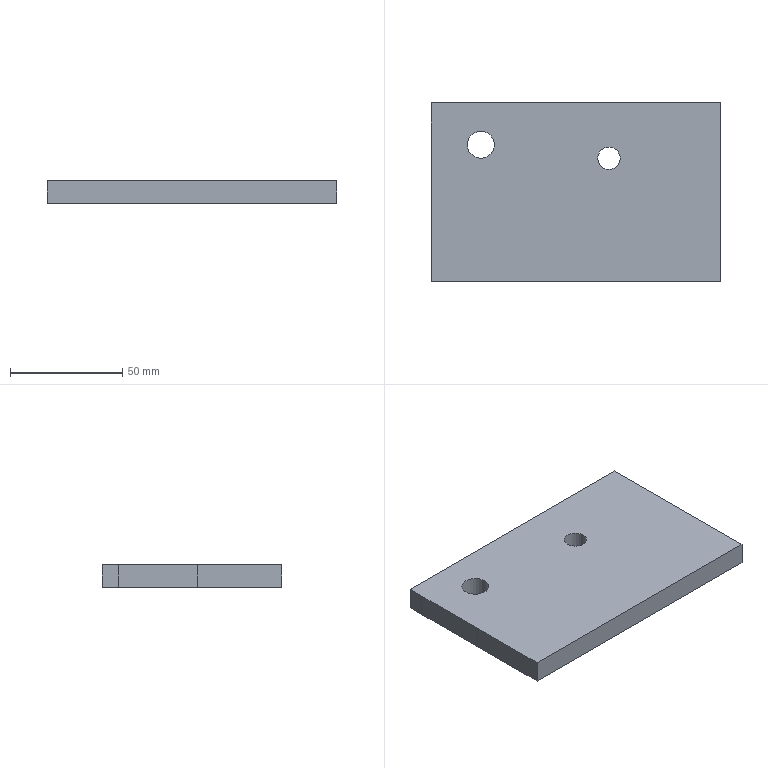Part | NX | features solid 2 | 1 solid | 10 faces | box 129 x 80 x 10 mm | volume 101284 mm3 | plane 8 | cylinder 2 | commonest cylinder face diameters 10 x1 12 x1
STEP:
#1=CARTESIAN_POINT('',(-398.,-109.,-5.));
#2=VERTEX_POINT('',#1);
#3=CARTESIAN_POINT('',(-392.,-109.,-5.));
#4=DIRECTION('',(0.,0.,-1.));
#5=DIRECTION('',(-1.,0.,0.));
#6=AXIS2_PLACEMENT_3D('',#3,#4,#5);
#7=CIRCLE('',#6,6.);
#8=EDGE_CURVE('',#2,#2,#7,.F.);
#9=ORIENTED_EDGE('',*,*,#8,.T.);
#10=EDGE_LOOP('',(#9));
#11=FACE_BOUND('',#10,.T.);
#12=CARTESIAN_POINT('',(-414.173,-170.,-5.));
#13=VERTEX_POINT('',#12);
#14=CARTESIAN_POINT('',(-285.173,-170.,-5.));
#15=VERTEX_POINT('',#14);
#16=CARTESIAN_POINT('',(-374.173,-170.,-5.));
#17=DIRECTION('',(-1.,0.,0.));
#18=VECTOR('',#17,1000.);
#19=LINE('',#16,#18);
#20=EDGE_CURVE('',#13,#15,#19,.F.);
#21=ORIENTED_EDGE('',*,*,#20,.F.);
#22=CARTESIAN_POINT('',(-414.173,-132.5,-5.));
#23=VERTEX_POINT('',#22);
#24=CARTESIAN_POINT('',(-414.173,-90.,-5.));
#25=DIRECTION('',(0.,-1.,0.));
#26=VECTOR('',#25,1000.);
#27=LINE('',#24,#26);
#28=EDGE_CURVE('',#23,#13,#27,.T.);
#29=ORIENTED_EDGE('',*,*,#28,.F.);
#30=CARTESIAN_POINT('',(-414.173,-97.5,-5.));
#31=VERTEX_POINT('',#30);
#32=CARTESIAN_POINT('',(-414.173,-90.,-5.));
#33=DIRECTION('',(0.,-1.,0.));
#34=VECTOR('',#33,1000.);
#35=LINE('',#32,#34);
#36=EDGE_CURVE('',#31,#23,#35,.T.);
#37=ORIENTED_EDGE('',*,*,#36,.F.);
#38=CARTESIAN_POINT('',(-414.173,-90.,-5.));
#39=VERTEX_POINT('',#38);
#40=CARTESIAN_POINT('',(-414.173,-90.,-5.));
#41=DIRECTION('',(0.,-1.,0.));
#42=VECTOR('',#41,1000.);
#43=LINE('',#40,#42);
#44=EDGE_CURVE('',#31,#39,#43,.F.);
#45=ORIENTED_EDGE('',*,*,#44,.T.);
#46=CARTESIAN_POINT('',(-285.173,-90.,-5.));
#47=VERTEX_POINT('',#46);
#48=CARTESIAN_POINT('',(-295.173,-90.,-5.));
#49=DIRECTION('',(-1.,0.,0.));
#50=VECTOR('',#49,1000.);
#51=LINE('',#48,#50);
#52=EDGE_CURVE('',#47,#39,#51,.T.);
#53=ORIENTED_EDGE('',*,*,#52,.F.);
#54=CARTESIAN_POINT('',(-285.173,-140.,-5.));
#55=DIRECTION('',(0.,1.,0.));
#56=VECTOR('',#55,1000.);
#57=LINE('',#54,#56);
#58=EDGE_CURVE('',#47,#15,#57,.F.);
#59=ORIENTED_EDGE('',*,*,#58,.T.);
#60=EDGE_LOOP('',(#21,#29,#37,#45,#53,#59));
#61=FACE_BOUND('',#60,.T.);
#62=CARTESIAN_POINT('',(-330.,-115.,-5.));
#63=VERTEX_POINT('',#62);
#64=CARTESIAN_POINT('',(-335.,-115.,-5.));
#65=DIRECTION('',(0.,0.,-1.));
#66=DIRECTION('',(1.,0.,0.));
#67=AXIS2_PLACEMENT_3D('',#64,#65,#66);
#68=CIRCLE('',#67,5.);
#69=EDGE_CURVE('',#63,#63,#68,.T.);
#70=ORIENTED_EDGE('',*,*,#69,.F.);
#71=EDGE_LOOP('',(#70));
#72=FACE_BOUND('',#71,.T.);
#73=CARTESIAN_POINT('',(-374.173,-140.,-5.));
#74=DIRECTION('',(0.,0.,-1.));
#75=DIRECTION('',(1.,0.,0.));
#76=AXIS2_PLACEMENT_3D('',#73,#74,#75);
#77=PLANE('',#76);
#78=ADVANCED_FACE('',(#11,#61,#72),#77,.T.);
#79=CARTESIAN_POINT('',(-398.,-109.,5.));
#80=VERTEX_POINT('',#79);
#81=CARTESIAN_POINT('',(-392.,-109.,5.));
#82=DIRECTION('',(0.,0.,-1.));
#83=DIRECTION('',(-1.,0.,0.));
#84=AXIS2_PLACEMENT_3D('',#81,#82,#83);
#85=CIRCLE('',#84,6.);
#86=EDGE_CURVE('',#80,#80,#85,.T.);
#87=ORIENTED_EDGE('',*,*,#86,.T.);
#88=EDGE_LOOP('',(#87));
#89=FACE_BOUND('',#88,.T.);
#90=CARTESIAN_POINT('',(-285.173,-170.,5.));
#91=VERTEX_POINT('',#90);
#92=CARTESIAN_POINT('',(-414.173,-170.,5.));
#93=VERTEX_POINT('',#92);
#94=CARTESIAN_POINT('',(-374.173,-170.,5.));
#95=DIRECTION('',(-1.,0.,0.));
#96=VECTOR('',#95,1000.);
#97=LINE('',#94,#96);
#98=EDGE_CURVE('',#91,#93,#97,.T.);
#99=ORIENTED_EDGE('',*,*,#98,.F.);
#100=CARTESIAN_POINT('',(-285.173,-90.,5.));
#101=VERTEX_POINT('',#100);
#102=CARTESIAN_POINT('',(-285.173,-140.,5.));
#103=DIRECTION('',(0.,1.,0.));
#104=VECTOR('',#103,1000.);
#105=LINE('',#102,#104);
#106=EDGE_CURVE('',#91,#101,#105,.T.);
#107=ORIENTED_EDGE('',*,*,#106,.T.);
#108=CARTESIAN_POINT('',(-414.173,-90.,5.));
#109=VERTEX_POINT('',#108);
#110=CARTESIAN_POINT('',(-295.173,-90.,5.));
#111=DIRECTION('',(-1.,0.,0.));
#112=VECTOR('',#111,1000.);
#113=LINE('',#110,#112);
#114=EDGE_CURVE('',#101,#109,#113,.T.);
#115=ORIENTED_EDGE('',*,*,#114,.T.);
#116=CARTESIAN_POINT('',(-414.173,-97.5,5.));
#117=VERTEX_POINT('',#116);
#118=CARTESIAN_POINT('',(-414.173,-140.,5.));
#119=DIRECTION('',(0.,1.,0.));
#120=VECTOR('',#119,1000.);
#121=LINE('',#118,#120);
#122=EDGE_CURVE('',#117,#109,#121,.T.);
#123=ORIENTED_EDGE('',*,*,#122,.F.);
#124=CARTESIAN_POINT('',(-414.173,-132.5,5.));
#125=VERTEX_POINT('',#124);
#126=CARTESIAN_POINT('',(-414.173,-140.,5.));
#127=DIRECTION('',(0.,1.,0.));
#128=VECTOR('',#127,1000.);
#129=LINE('',#126,#128);
#130=EDGE_CURVE('',#117,#125,#129,.F.);
#131=ORIENTED_EDGE('',*,*,#130,.T.);
#132=CARTESIAN_POINT('',(-414.173,-140.,5.));
#133=DIRECTION('',(0.,1.,0.));
#134=VECTOR('',#133,1000.);
#135=LINE('',#132,#134);
#136=EDGE_CURVE('',#125,#93,#135,.F.);
#137=ORIENTED_EDGE('',*,*,#136,.T.);
#138=EDGE_LOOP('',(#99,#107,#115,#123,#131,#137));
#139=FACE_BOUND('',#138,.T.);
#140=CARTESIAN_POINT('',(-340.,-115.,5.));
#141=VERTEX_POINT('',#140);
#142=CARTESIAN_POINT('',(-335.,-115.,5.));
#143=DIRECTION('',(0.,0.,-1.));
#144=DIRECTION('',(-1.,0.,0.));
#145=AXIS2_PLACEMENT_3D('',#142,#143,#144);
#146=CIRCLE('',#145,5.);
#147=EDGE_CURVE('',#141,#141,#146,.T.);
#148=ORIENTED_EDGE('',*,*,#147,.T.);
#149=EDGE_LOOP('',(#148));
#150=FACE_BOUND('',#149,.T.);
#151=CARTESIAN_POINT('',(-374.173,-140.,5.));
#152=DIRECTION('',(0.,0.,-1.));
#153=DIRECTION('',(1.,0.,0.));
#154=AXIS2_PLACEMENT_3D('',#151,#152,#153);
#155=PLANE('',#154);
#156=ADVANCED_FACE('',(#89,#139,#150),#155,.F.);
#157=ORIENTED_EDGE('',*,*,#106,.F.);
#158=CARTESIAN_POINT('',(-285.173,-170.,-35.));
#159=DIRECTION('',(0.,0.,1.));
#160=VECTOR('',#159,1000.);
#161=LINE('',#158,#160);
#162=EDGE_CURVE('',#15,#91,#161,.T.);
#163=ORIENTED_EDGE('',*,*,#162,.F.);
#164=ORIENTED_EDGE('',*,*,#58,.F.);
#165=CARTESIAN_POINT('',(-285.173,-90.,-5.));
#166=DIRECTION('',(0.,0.,-1.));
#167=VECTOR('',#166,1000.);
#168=LINE('',#165,#167);
#169=EDGE_CURVE('',#47,#101,#168,.F.);
#170=ORIENTED_EDGE('',*,*,#169,.T.);
#171=EDGE_LOOP('',(#157,#163,#164,#170));
#172=FACE_BOUND('',#171,.T.);
#173=CARTESIAN_POINT('',(-285.173,-140.,-5.));
#174=DIRECTION('',(1.,0.,0.));
#175=DIRECTION('',(0.,1.,0.));
#176=AXIS2_PLACEMENT_3D('',#173,#174,#175);
#177=PLANE('',#176);
#178=ADVANCED_FACE('',(#172),#177,.T.);
#179=ORIENTED_EDGE('',*,*,#130,.F.);
#180=CARTESIAN_POINT('',(-414.173,-97.5,-5.));
#181=DIRECTION('',(0.,0.,1.));
#182=VECTOR('',#181,1000.);
#183=LINE('',#180,#182);
#184=EDGE_CURVE('',#31,#117,#183,.T.);
#185=ORIENTED_EDGE('',*,*,#184,.F.);
#186=ORIENTED_EDGE('',*,*,#36,.T.);
#187=CARTESIAN_POINT('',(-414.173,-132.5,-5.));
#188=DIRECTION('',(0.,0.,1.));
#189=VECTOR('',#188,1000.);
#190=LINE('',#187,#189);
#191=EDGE_CURVE('',#23,#125,#190,.T.);
#192=ORIENTED_EDGE('',*,*,#191,.T.);
#193=EDGE_LOOP('',(#179,#185,#186,#192));
#194=FACE_BOUND('',#193,.T.);
#195=CARTESIAN_POINT('',(-414.173,-90.,-5.));
#196=DIRECTION('',(-1.,0.,0.));
#197=DIRECTION('',(0.,-1.,0.));
#198=AXIS2_PLACEMENT_3D('',#195,#196,#197);
#199=PLANE('',#198);
#200=ADVANCED_FACE('',(#194),#199,.T.);
#201=ORIENTED_EDGE('',*,*,#136,.F.);
#202=ORIENTED_EDGE('',*,*,#191,.F.);
#203=ORIENTED_EDGE('',*,*,#28,.T.);
#204=CARTESIAN_POINT('',(-414.173,-170.,-35.));
#205=DIRECTION('',(0.,0.,-1.));
#206=VECTOR('',#205,1000.);
#207=LINE('',#204,#206);
#208=EDGE_CURVE('',#13,#93,#207,.F.);
#209=ORIENTED_EDGE('',*,*,#208,.T.);
#210=EDGE_LOOP('',(#201,#202,#203,#209));
#211=FACE_BOUND('',#210,.T.);
#212=CARTESIAN_POINT('',(-414.173,-90.,-5.));
#213=DIRECTION('',(-1.,0.,0.));
#214=DIRECTION('',(0.,-1.,0.));
#215=AXIS2_PLACEMENT_3D('',#212,#213,#214);
#216=PLANE('',#215);
#217=ADVANCED_FACE('',(#211),#216,.T.);
#218=ORIENTED_EDGE('',*,*,#114,.F.);
#219=ORIENTED_EDGE('',*,*,#169,.F.);
#220=ORIENTED_EDGE('',*,*,#52,.T.);
#221=CARTESIAN_POINT('',(-414.173,-90.,-5.));
#222=DIRECTION('',(0.,0.,-1.));
#223=VECTOR('',#222,1000.);
#224=LINE('',#221,#223);
#225=EDGE_CURVE('',#39,#109,#224,.F.);
#226=ORIENTED_EDGE('',*,*,#225,.T.);
#227=EDGE_LOOP('',(#218,#219,#220,#226));
#228=FACE_BOUND('',#227,.T.);
#229=CARTESIAN_POINT('',(-295.173,-90.,-5.));
#230=DIRECTION('',(0.,1.,0.));
#231=DIRECTION('',(-1.,0.,0.));
#232=AXIS2_PLACEMENT_3D('',#229,#230,#231);
#233=PLANE('',#232);
#234=ADVANCED_FACE('',(#228),#233,.T.);
#235=ORIENTED_EDGE('',*,*,#122,.T.);
#236=ORIENTED_EDGE('',*,*,#225,.F.);
#237=ORIENTED_EDGE('',*,*,#44,.F.);
#238=ORIENTED_EDGE('',*,*,#184,.T.);
#239=EDGE_LOOP('',(#235,#236,#237,#238));
#240=FACE_BOUND('',#239,.T.);
#241=CARTESIAN_POINT('',(-414.173,-90.,-5.));
#242=DIRECTION('',(-1.,0.,0.));
#243=DIRECTION('',(0.,-1.,0.));
#244=AXIS2_PLACEMENT_3D('',#241,#242,#243);
#245=PLANE('',#244);
#246=ADVANCED_FACE('',(#240),#245,.T.);
#247=ORIENTED_EDGE('',*,*,#8,.F.);
#248=EDGE_LOOP('',(#247));
#249=FACE_BOUND('',#248,.T.);
#250=ORIENTED_EDGE('',*,*,#86,.F.);
#251=EDGE_LOOP('',(#250));
#252=FACE_BOUND('',#251,.T.);
#253=CARTESIAN_POINT('',(-392.,-109.,70.));
#254=DIRECTION('',(0.,0.,-1.));
#255=DIRECTION('',(1.,0.,0.));
#256=AXIS2_PLACEMENT_3D('',#253,#254,#255);
#257=CYLINDRICAL_SURFACE('',#256,6.);
#258=ADVANCED_FACE('',(#249,#252),#257,.F.);
#259=ORIENTED_EDGE('',*,*,#20,.T.);
#260=ORIENTED_EDGE('',*,*,#162,.T.);
#261=ORIENTED_EDGE('',*,*,#98,.T.);
#262=ORIENTED_EDGE('',*,*,#208,.F.);
#263=EDGE_LOOP('',(#259,#260,#261,#262));
#264=FACE_BOUND('',#263,.T.);
#265=CARTESIAN_POINT('',(-374.173,-170.,-35.));
#266=DIRECTION('',(0.,-1.,0.));
#267=DIRECTION('',(0.,0.,-1.));
#268=AXIS2_PLACEMENT_3D('',#265,#266,#267);
#269=PLANE('',#268);
#270=ADVANCED_FACE('',(#264),#269,.T.);
#271=ORIENTED_EDGE('',*,*,#147,.F.);
#272=EDGE_LOOP('',(#271));
#273=FACE_BOUND('',#272,.T.);
#274=ORIENTED_EDGE('',*,*,#69,.T.);
#275=EDGE_LOOP('',(#274));
#276=FACE_BOUND('',#275,.T.);
#277=CARTESIAN_POINT('',(-335.,-115.,-5.));
#278=DIRECTION('',(0.,0.,1.));
#279=DIRECTION('',(1.,0.,0.));
#280=AXIS2_PLACEMENT_3D('',#277,#278,#279);
#281=CYLINDRICAL_SURFACE('',#280,5.);
#282=ADVANCED_FACE('',(#273,#276),#281,.F.);
#283=CLOSED_SHELL('',(#78,#156,#178,#200,#217,#234,#246,#258,#270,#282));
#284=MANIFOLD_SOLID_BREP('',#283);
#285=(LENGTH_UNIT()NAMED_UNIT(*)SI_UNIT(.MILLI.,.METRE.));
#286=UNCERTAINTY_MEASURE_WITH_UNIT(LENGTH_MEASURE(0.00001),#285,'','');
#287=(NAMED_UNIT(*)PLANE_ANGLE_UNIT()SI_UNIT($,.RADIAN.));
#288=(NAMED_UNIT(*)SI_UNIT($,.STERADIAN.)SOLID_ANGLE_UNIT());
#289=(GEOMETRIC_REPRESENTATION_CONTEXT(3)GLOBAL_UNCERTAINTY_ASSIGNED_CONTEXT((#286))GLOBAL_UNIT_ASSIGNED_CONTEXT((#285,#287,#288))REPRESENTATION_CONTEXT('',''));
#290=ADVANCED_BREP_SHAPE_REPRESENTATION('',(#284),#289);